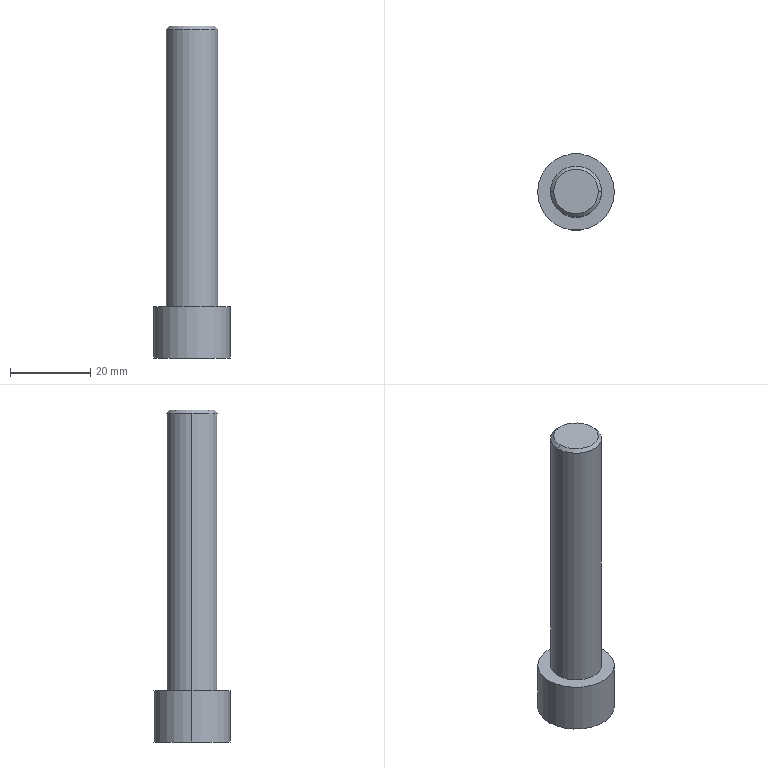Part | STEP file | 4-20.sldasm-Part-357 | 1 solid | 16 faces | box 19.05 x 19.05 x 82.55 mm | volume 11798 mm3 | plane 10 | cylinder 4 | cone 2 | commonest cylinder face diameters 12.7 x2 19.05 x2
STEP:
#1=CARTESIAN_POINT('',(90.556,-50.,63.312));
#2=VERTEX_POINT('',#1);
#3=CARTESIAN_POINT('',(79.444,-50.,63.312));
#4=VERTEX_POINT('',#3);
#5=CARTESIAN_POINT('',(85.,-50.,63.312));
#6=DIRECTION('',(0.,0.,1.));
#7=DIRECTION('',(-1.,0.,0.));
#8=AXIS2_PLACEMENT_3D('',#5,#6,#7);
#9=CIRCLE('',#8,5.556);
#10=EDGE_CURVE('',#2,#4,#9,.T.);
#11=ORIENTED_EDGE('',*,*,#10,.F.);
#12=CARTESIAN_POINT('',(91.35,-50.,62.518));
#13=VERTEX_POINT('',#12);
#14=CARTESIAN_POINT('',(91.35,-50.,62.518));
#15=DIRECTION('',(0.7071,0.,-0.7071));
#16=VECTOR('',#15,1000.);
#17=LINE('',#14,#16);
#18=EDGE_CURVE('',#2,#13,#17,.T.);
#19=ORIENTED_EDGE('',*,*,#18,.T.);
#20=CARTESIAN_POINT('',(78.65,-50.,62.518));
#21=VERTEX_POINT('',#20);
#22=CARTESIAN_POINT('',(85.,-50.,62.518));
#23=DIRECTION('',(0.,0.,-1.));
#24=DIRECTION('',(-1.,0.,0.));
#25=AXIS2_PLACEMENT_3D('',#22,#23,#24);
#26=CIRCLE('',#25,6.35);
#27=EDGE_CURVE('',#21,#13,#26,.T.);
#28=ORIENTED_EDGE('',*,*,#27,.F.);
#29=CARTESIAN_POINT('',(78.65,-50.,62.518));
#30=DIRECTION('',(-0.7071,0.,-0.7071));
#31=VECTOR('',#30,1000.);
#32=LINE('',#29,#31);
#33=EDGE_CURVE('',#4,#21,#32,.T.);
#34=ORIENTED_EDGE('',*,*,#33,.F.);
#35=EDGE_LOOP('',(#11,#19,#28,#34));
#36=FACE_OUTER_BOUND('',#35,.T.);
#37=CARTESIAN_POINT('',(85.,-50.,62.518));
#38=DIRECTION('',(0.,0.,-1.));
#39=DIRECTION('',(-1.,0.,0.));
#40=AXIS2_PLACEMENT_3D('',#37,#38,#39);
#41=CONICAL_SURFACE('',#40,6.35,0.7854);
#42=ADVANCED_FACE('',(#36),#41,.T.);
#43=CARTESIAN_POINT('',(75.475,-50.,-6.538));
#44=VERTEX_POINT('',#43);
#45=CARTESIAN_POINT('',(94.525,-50.,-6.538));
#46=VERTEX_POINT('',#45);
#47=CARTESIAN_POINT('',(85.,-50.,-6.538));
#48=DIRECTION('',(0.,0.,-1.));
#49=DIRECTION('',(-1.,0.,0.));
#50=AXIS2_PLACEMENT_3D('',#47,#48,#49);
#51=CIRCLE('',#50,9.525);
#52=EDGE_CURVE('',#44,#46,#51,.T.);
#53=ORIENTED_EDGE('',*,*,#52,.T.);
#54=CARTESIAN_POINT('',(94.525,-50.,-19.238));
#55=VERTEX_POINT('',#54);
#56=CARTESIAN_POINT('',(94.525,-50.,-6.538));
#57=DIRECTION('',(0.,0.,-1.));
#58=VECTOR('',#57,1000.);
#59=LINE('',#56,#58);
#60=EDGE_CURVE('',#46,#55,#59,.T.);
#61=ORIENTED_EDGE('',*,*,#60,.T.);
#62=CARTESIAN_POINT('',(75.475,-50.,-19.238));
#63=VERTEX_POINT('',#62);
#64=CARTESIAN_POINT('',(85.,-50.,-19.238));
#65=DIRECTION('',(0.,0.,-1.));
#66=DIRECTION('',(-1.,0.,0.));
#67=AXIS2_PLACEMENT_3D('',#64,#65,#66);
#68=CIRCLE('',#67,9.525);
#69=EDGE_CURVE('',#63,#55,#68,.T.);
#70=ORIENTED_EDGE('',*,*,#69,.F.);
#71=CARTESIAN_POINT('',(75.475,-50.,-6.538));
#72=DIRECTION('',(0.,0.,-1.));
#73=VECTOR('',#72,1000.);
#74=LINE('',#71,#73);
#75=EDGE_CURVE('',#44,#63,#74,.T.);
#76=ORIENTED_EDGE('',*,*,#75,.F.);
#77=EDGE_LOOP('',(#53,#61,#70,#76));
#78=FACE_OUTER_BOUND('',#77,.T.);
#79=CARTESIAN_POINT('',(85.,-50.,-6.538));
#80=DIRECTION('',(0.,0.,-1.));
#81=DIRECTION('',(-1.,0.,0.));
#82=AXIS2_PLACEMENT_3D('',#79,#80,#81);
#83=CYLINDRICAL_SURFACE('',#82,9.525);
#84=ADVANCED_FACE('',(#78),#83,.T.);
#85=CARTESIAN_POINT('',(78.65,-50.,-6.538));
#86=VERTEX_POINT('',#85);
#87=CARTESIAN_POINT('',(91.35,-50.,-6.538));
#88=VERTEX_POINT('',#87);
#89=CARTESIAN_POINT('',(85.,-50.,-6.538));
#90=DIRECTION('',(0.,0.,-1.));
#91=DIRECTION('',(-1.,0.,0.));
#92=AXIS2_PLACEMENT_3D('',#89,#90,#91);
#93=CIRCLE('',#92,6.35);
#94=EDGE_CURVE('',#86,#88,#93,.T.);
#95=ORIENTED_EDGE('',*,*,#94,.F.);
#96=CARTESIAN_POINT('',(78.65,-50.,-6.538));
#97=DIRECTION('',(0.,0.,1.));
#98=VECTOR('',#97,1000.);
#99=LINE('',#96,#98);
#100=EDGE_CURVE('',#86,#21,#99,.T.);
#101=ORIENTED_EDGE('',*,*,#100,.T.);
#102=ORIENTED_EDGE('',*,*,#27,.T.);
#103=CARTESIAN_POINT('',(91.35,-50.,-6.538));
#104=DIRECTION('',(0.,0.,1.));
#105=VECTOR('',#104,1000.);
#106=LINE('',#103,#105);
#107=EDGE_CURVE('',#88,#13,#106,.T.);
#108=ORIENTED_EDGE('',*,*,#107,.F.);
#109=EDGE_LOOP('',(#95,#101,#102,#108));
#110=FACE_OUTER_BOUND('',#109,.T.);
#111=CARTESIAN_POINT('',(85.,-50.,-6.538));
#112=DIRECTION('',(0.,0.,1.));
#113=DIRECTION('',(1.,0.,0.));
#114=AXIS2_PLACEMENT_3D('',#111,#112,#113);
#115=CYLINDRICAL_SURFACE('',#114,6.35);
#116=ADVANCED_FACE('',(#110),#115,.T.);
#117=ORIENTED_EDGE('',*,*,#100,.F.);
#118=CARTESIAN_POINT('',(85.,-50.,-6.538));
#119=DIRECTION('',(0.,0.,-1.));
#120=DIRECTION('',(-1.,0.,0.));
#121=AXIS2_PLACEMENT_3D('',#118,#119,#120);
#122=CIRCLE('',#121,6.35);
#123=EDGE_CURVE('',#88,#86,#122,.T.);
#124=ORIENTED_EDGE('',*,*,#123,.F.);
#125=ORIENTED_EDGE('',*,*,#107,.T.);
#126=CARTESIAN_POINT('',(85.,-50.,62.518));
#127=DIRECTION('',(0.,0.,-1.));
#128=DIRECTION('',(-1.,0.,0.));
#129=AXIS2_PLACEMENT_3D('',#126,#127,#128);
#130=CIRCLE('',#129,6.35);
#131=EDGE_CURVE('',#13,#21,#130,.T.);
#132=ORIENTED_EDGE('',*,*,#131,.T.);
#133=EDGE_LOOP('',(#117,#124,#125,#132));
#134=FACE_OUTER_BOUND('',#133,.T.);
#135=CARTESIAN_POINT('',(85.,-50.,-6.538));
#136=DIRECTION('',(0.,0.,1.));
#137=DIRECTION('',(1.,0.,0.));
#138=AXIS2_PLACEMENT_3D('',#135,#136,#137);
#139=CYLINDRICAL_SURFACE('',#138,6.35);
#140=ADVANCED_FACE('',(#134),#139,.T.);
#141=CARTESIAN_POINT('',(85.,-50.,63.312));
#142=DIRECTION('',(0.,0.,1.));
#143=DIRECTION('',(-1.,0.,0.));
#144=AXIS2_PLACEMENT_3D('',#141,#142,#143);
#145=CIRCLE('',#144,5.556);
#146=EDGE_CURVE('',#4,#2,#145,.T.);
#147=ORIENTED_EDGE('',*,*,#146,.T.);
#148=ORIENTED_EDGE('',*,*,#10,.T.);
#149=EDGE_LOOP('',(#147,#148));
#150=FACE_OUTER_BOUND('',#149,.T.);
#151=CARTESIAN_POINT('',(85.,-50.,63.312));
#152=DIRECTION('',(0.,0.,-1.));
#153=DIRECTION('',(-1.,0.,0.));
#154=AXIS2_PLACEMENT_3D('',#151,#152,#153);
#155=PLANE('',#154);
#156=ADVANCED_FACE('',(#150),#155,.F.);
#157=ORIENTED_EDGE('',*,*,#52,.F.);
#158=CARTESIAN_POINT('',(85.,-50.,-6.538));
#159=DIRECTION('',(0.,0.,-1.));
#160=DIRECTION('',(-1.,0.,0.));
#161=AXIS2_PLACEMENT_3D('',#158,#159,#160);
#162=CIRCLE('',#161,9.525);
#163=EDGE_CURVE('',#46,#44,#162,.T.);
#164=ORIENTED_EDGE('',*,*,#163,.F.);
#165=EDGE_LOOP('',(#157,#164));
#166=FACE_OUTER_BOUND('',#165,.T.);
#167=ORIENTED_EDGE('',*,*,#123,.T.);
#168=ORIENTED_EDGE('',*,*,#94,.T.);
#169=EDGE_LOOP('',(#167,#168));
#170=FACE_BOUND('',#169,.T.);
#171=CARTESIAN_POINT('',(85.,-50.,-6.538));
#172=DIRECTION('',(0.,0.,1.));
#173=DIRECTION('',(1.,0.,0.));
#174=AXIS2_PLACEMENT_3D('',#171,#172,#173);
#175=PLANE('',#174);
#176=ADVANCED_FACE('',(#166,#170),#175,.T.);
#177=CARTESIAN_POINT('',(87.75,-54.763,-19.238));
#178=VERTEX_POINT('',#177);
#179=CARTESIAN_POINT('',(82.25,-54.763,-19.238));
#180=VERTEX_POINT('',#179);
#181=CARTESIAN_POINT('',(87.75,-54.763,-19.238));
#182=DIRECTION('',(-1.,0.,0.));
#183=VECTOR('',#182,1000.);
#184=LINE('',#181,#183);
#185=EDGE_CURVE('',#178,#180,#184,.T.);
#186=ORIENTED_EDGE('',*,*,#185,.F.);
#187=CARTESIAN_POINT('',(90.499,-50.,-19.238));
#188=VERTEX_POINT('',#187);
#189=CARTESIAN_POINT('',(90.499,-50.,-19.238));
#190=DIRECTION('',(-0.5,-0.866,0.));
#191=VECTOR('',#190,1000.);
#192=LINE('',#189,#191);
#193=EDGE_CURVE('',#188,#178,#192,.T.);
#194=ORIENTED_EDGE('',*,*,#193,.F.);
#195=CARTESIAN_POINT('',(87.75,-45.238,-19.238));
#196=VERTEX_POINT('',#195);
#197=CARTESIAN_POINT('',(87.75,-45.238,-19.238));
#198=DIRECTION('',(0.5,-0.866,0.));
#199=VECTOR('',#198,1000.);
#200=LINE('',#197,#199);
#201=EDGE_CURVE('',#196,#188,#200,.T.);
#202=ORIENTED_EDGE('',*,*,#201,.F.);
#203=CARTESIAN_POINT('',(82.25,-45.238,-19.238));
#204=VERTEX_POINT('',#203);
#205=CARTESIAN_POINT('',(82.25,-45.238,-19.238));
#206=DIRECTION('',(1.,0.,0.));
#207=VECTOR('',#206,1000.);
#208=LINE('',#205,#207);
#209=EDGE_CURVE('',#204,#196,#208,.T.);
#210=ORIENTED_EDGE('',*,*,#209,.F.);
#211=CARTESIAN_POINT('',(79.501,-50.,-19.238));
#212=VERTEX_POINT('',#211);
#213=CARTESIAN_POINT('',(79.501,-50.,-19.238));
#214=DIRECTION('',(0.5,0.866,0.));
#215=VECTOR('',#214,1000.);
#216=LINE('',#213,#215);
#217=EDGE_CURVE('',#212,#204,#216,.T.);
#218=ORIENTED_EDGE('',*,*,#217,.F.);
#219=CARTESIAN_POINT('',(82.25,-54.763,-19.238));
#220=DIRECTION('',(-0.5,0.866,0.));
#221=VECTOR('',#220,1000.);
#222=LINE('',#219,#221);
#223=EDGE_CURVE('',#180,#212,#222,.T.);
#224=ORIENTED_EDGE('',*,*,#223,.F.);
#225=EDGE_LOOP('',(#186,#194,#202,#210,#218,#224));
#226=FACE_BOUND('',#225,.T.);
#227=ORIENTED_EDGE('',*,*,#69,.T.);
#228=CARTESIAN_POINT('',(85.,-50.,-19.238));
#229=DIRECTION('',(0.,0.,-1.));
#230=DIRECTION('',(-1.,0.,0.));
#231=AXIS2_PLACEMENT_3D('',#228,#229,#230);
#232=CIRCLE('',#231,9.525);
#233=EDGE_CURVE('',#55,#63,#232,.T.);
#234=ORIENTED_EDGE('',*,*,#233,.T.);
#235=EDGE_LOOP('',(#227,#234));
#236=FACE_OUTER_BOUND('',#235,.T.);
#237=CARTESIAN_POINT('',(85.,-50.,-19.238));
#238=DIRECTION('',(0.,0.,-1.));
#239=DIRECTION('',(-1.,0.,0.));
#240=AXIS2_PLACEMENT_3D('',#237,#238,#239);
#241=PLANE('',#240);
#242=ADVANCED_FACE('',(#226,#236),#241,.T.);
#243=ORIENTED_EDGE('',*,*,#60,.F.);
#244=ORIENTED_EDGE('',*,*,#163,.T.);
#245=ORIENTED_EDGE('',*,*,#75,.T.);
#246=ORIENTED_EDGE('',*,*,#233,.F.);
#247=EDGE_LOOP('',(#243,#244,#245,#246));
#248=FACE_OUTER_BOUND('',#247,.T.);
#249=CARTESIAN_POINT('',(85.,-50.,-6.538));
#250=DIRECTION('',(0.,0.,-1.));
#251=DIRECTION('',(-1.,0.,0.));
#252=AXIS2_PLACEMENT_3D('',#249,#250,#251);
#253=CYLINDRICAL_SURFACE('',#252,9.525);
#254=ADVANCED_FACE('',(#248),#253,.T.);
#255=ORIENTED_EDGE('',*,*,#18,.F.);
#256=ORIENTED_EDGE('',*,*,#146,.F.);
#257=ORIENTED_EDGE('',*,*,#33,.T.);
#258=ORIENTED_EDGE('',*,*,#131,.F.);
#259=EDGE_LOOP('',(#255,#256,#257,#258));
#260=FACE_OUTER_BOUND('',#259,.T.);
#261=CARTESIAN_POINT('',(85.,-50.,62.518));
#262=DIRECTION('',(0.,0.,-1.));
#263=DIRECTION('',(-1.,0.,0.));
#264=AXIS2_PLACEMENT_3D('',#261,#262,#263);
#265=CONICAL_SURFACE('',#264,6.35,0.7854);
#266=ADVANCED_FACE('',(#260),#265,.T.);
#267=ORIENTED_EDGE('',*,*,#185,.T.);
#268=CARTESIAN_POINT('',(82.25,-54.763,-10.856));
#269=VERTEX_POINT('',#268);
#270=CARTESIAN_POINT('',(82.25,-54.763,-10.856));
#271=DIRECTION('',(0.,0.,-1.));
#272=VECTOR('',#271,1000.);
#273=LINE('',#270,#272);
#274=EDGE_CURVE('',#269,#180,#273,.T.);
#275=ORIENTED_EDGE('',*,*,#274,.F.);
#276=CARTESIAN_POINT('',(87.75,-54.763,-10.856));
#277=VERTEX_POINT('',#276);
#278=CARTESIAN_POINT('',(87.75,-54.763,-10.856));
#279=DIRECTION('',(-1.,0.,0.));
#280=VECTOR('',#279,1000.);
#281=LINE('',#278,#280);
#282=EDGE_CURVE('',#277,#269,#281,.T.);
#283=ORIENTED_EDGE('',*,*,#282,.F.);
#284=CARTESIAN_POINT('',(87.75,-54.763,-10.856));
#285=DIRECTION('',(0.,0.,-1.));
#286=VECTOR('',#285,1000.);
#287=LINE('',#284,#286);
#288=EDGE_CURVE('',#277,#178,#287,.T.);
#289=ORIENTED_EDGE('',*,*,#288,.T.);
#290=EDGE_LOOP('',(#267,#275,#283,#289));
#291=FACE_OUTER_BOUND('',#290,.T.);
#292=CARTESIAN_POINT('',(87.75,-54.763,-10.856));
#293=DIRECTION('',(0.,-1.,0.));
#294=DIRECTION('',(0.,0.,1.));
#295=AXIS2_PLACEMENT_3D('',#292,#293,#294);
#296=PLANE('',#295);
#297=ADVANCED_FACE('',(#291),#296,.F.);
#298=ORIENTED_EDGE('',*,*,#223,.T.);
#299=CARTESIAN_POINT('',(79.501,-50.,-10.856));
#300=VERTEX_POINT('',#299);
#301=CARTESIAN_POINT('',(79.501,-50.,-10.856));
#302=DIRECTION('',(0.,0.,-1.));
#303=VECTOR('',#302,1000.);
#304=LINE('',#301,#303);
#305=EDGE_CURVE('',#300,#212,#304,.T.);
#306=ORIENTED_EDGE('',*,*,#305,.F.);
#307=CARTESIAN_POINT('',(82.25,-54.763,-10.856));
#308=DIRECTION('',(-0.5,0.866,0.));
#309=VECTOR('',#308,1000.);
#310=LINE('',#307,#309);
#311=EDGE_CURVE('',#269,#300,#310,.T.);
#312=ORIENTED_EDGE('',*,*,#311,.F.);
#313=ORIENTED_EDGE('',*,*,#274,.T.);
#314=EDGE_LOOP('',(#298,#306,#312,#313));
#315=FACE_OUTER_BOUND('',#314,.T.);
#316=CARTESIAN_POINT('',(82.25,-54.763,-10.856));
#317=DIRECTION('',(-0.866,-0.5,0.));
#318=DIRECTION('',(-0.5,0.866,0.));
#319=AXIS2_PLACEMENT_3D('',#316,#317,#318);
#320=PLANE('',#319);
#321=ADVANCED_FACE('',(#315),#320,.F.);
#322=ORIENTED_EDGE('',*,*,#217,.T.);
#323=CARTESIAN_POINT('',(82.25,-45.238,-10.856));
#324=VERTEX_POINT('',#323);
#325=CARTESIAN_POINT('',(82.25,-45.238,-10.856));
#326=DIRECTION('',(0.,0.,-1.));
#327=VECTOR('',#326,1000.);
#328=LINE('',#325,#327);
#329=EDGE_CURVE('',#324,#204,#328,.T.);
#330=ORIENTED_EDGE('',*,*,#329,.F.);
#331=CARTESIAN_POINT('',(79.501,-50.,-10.856));
#332=DIRECTION('',(0.5,0.866,0.));
#333=VECTOR('',#332,1000.);
#334=LINE('',#331,#333);
#335=EDGE_CURVE('',#300,#324,#334,.T.);
#336=ORIENTED_EDGE('',*,*,#335,.F.);
#337=ORIENTED_EDGE('',*,*,#305,.T.);
#338=EDGE_LOOP('',(#322,#330,#336,#337));
#339=FACE_OUTER_BOUND('',#338,.T.);
#340=CARTESIAN_POINT('',(79.501,-50.,-10.856));
#341=DIRECTION('',(-0.866,0.5,0.));
#342=DIRECTION('',(0.5,0.866,0.));
#343=AXIS2_PLACEMENT_3D('',#340,#341,#342);
#344=PLANE('',#343);
#345=ADVANCED_FACE('',(#339),#344,.F.);
#346=ORIENTED_EDGE('',*,*,#209,.T.);
#347=CARTESIAN_POINT('',(87.75,-45.238,-10.856));
#348=VERTEX_POINT('',#347);
#349=CARTESIAN_POINT('',(87.75,-45.238,-10.856));
#350=DIRECTION('',(0.,0.,-1.));
#351=VECTOR('',#350,1000.);
#352=LINE('',#349,#351);
#353=EDGE_CURVE('',#348,#196,#352,.T.);
#354=ORIENTED_EDGE('',*,*,#353,.F.);
#355=CARTESIAN_POINT('',(82.25,-45.238,-10.856));
#356=DIRECTION('',(1.,0.,0.));
#357=VECTOR('',#356,1000.);
#358=LINE('',#355,#357);
#359=EDGE_CURVE('',#324,#348,#358,.T.);
#360=ORIENTED_EDGE('',*,*,#359,.F.);
#361=ORIENTED_EDGE('',*,*,#329,.T.);
#362=EDGE_LOOP('',(#346,#354,#360,#361));
#363=FACE_OUTER_BOUND('',#362,.T.);
#364=CARTESIAN_POINT('',(82.25,-45.238,-10.856));
#365=DIRECTION('',(0.,1.,0.));
#366=DIRECTION('',(0.,0.,-1.));
#367=AXIS2_PLACEMENT_3D('',#364,#365,#366);
#368=PLANE('',#367);
#369=ADVANCED_FACE('',(#363),#368,.F.);
#370=ORIENTED_EDGE('',*,*,#201,.T.);
#371=CARTESIAN_POINT('',(90.499,-50.,-10.856));
#372=VERTEX_POINT('',#371);
#373=CARTESIAN_POINT('',(90.499,-50.,-10.856));
#374=DIRECTION('',(0.,0.,-1.));
#375=VECTOR('',#374,1000.);
#376=LINE('',#373,#375);
#377=EDGE_CURVE('',#372,#188,#376,.T.);
#378=ORIENTED_EDGE('',*,*,#377,.F.);
#379=CARTESIAN_POINT('',(87.75,-45.238,-10.856));
#380=DIRECTION('',(0.5,-0.866,0.));
#381=VECTOR('',#380,1000.);
#382=LINE('',#379,#381);
#383=EDGE_CURVE('',#348,#372,#382,.T.);
#384=ORIENTED_EDGE('',*,*,#383,.F.);
#385=ORIENTED_EDGE('',*,*,#353,.T.);
#386=EDGE_LOOP('',(#370,#378,#384,#385));
#387=FACE_OUTER_BOUND('',#386,.T.);
#388=CARTESIAN_POINT('',(87.75,-45.238,-10.856));
#389=DIRECTION('',(0.866,0.5,0.));
#390=DIRECTION('',(0.5,-0.866,0.));
#391=AXIS2_PLACEMENT_3D('',#388,#389,#390);
#392=PLANE('',#391);
#393=ADVANCED_FACE('',(#387),#392,.F.);
#394=ORIENTED_EDGE('',*,*,#193,.T.);
#395=ORIENTED_EDGE('',*,*,#288,.F.);
#396=CARTESIAN_POINT('',(90.499,-50.,-10.856));
#397=DIRECTION('',(-0.5,-0.866,0.));
#398=VECTOR('',#397,1000.);
#399=LINE('',#396,#398);
#400=EDGE_CURVE('',#372,#277,#399,.T.);
#401=ORIENTED_EDGE('',*,*,#400,.F.);
#402=ORIENTED_EDGE('',*,*,#377,.T.);
#403=EDGE_LOOP('',(#394,#395,#401,#402));
#404=FACE_OUTER_BOUND('',#403,.T.);
#405=CARTESIAN_POINT('',(90.499,-50.,-10.856));
#406=DIRECTION('',(0.866,-0.5,0.));
#407=DIRECTION('',(-0.5,-0.866,0.));
#408=AXIS2_PLACEMENT_3D('',#405,#406,#407);
#409=PLANE('',#408);
#410=ADVANCED_FACE('',(#404),#409,.F.);
#411=ORIENTED_EDGE('',*,*,#282,.T.);
#412=ORIENTED_EDGE('',*,*,#311,.T.);
#413=ORIENTED_EDGE('',*,*,#335,.T.);
#414=ORIENTED_EDGE('',*,*,#359,.T.);
#415=ORIENTED_EDGE('',*,*,#383,.T.);
#416=ORIENTED_EDGE('',*,*,#400,.T.);
#417=EDGE_LOOP('',(#411,#412,#413,#414,#415,#416));
#418=FACE_OUTER_BOUND('',#417,.T.);
#419=CARTESIAN_POINT('',(82.25,-54.763,-10.856));
#420=DIRECTION('',(0.,0.,-1.));
#421=DIRECTION('',(-1.,0.,0.));
#422=AXIS2_PLACEMENT_3D('',#419,#420,#421);
#423=PLANE('',#422);
#424=ADVANCED_FACE('',(#418),#423,.T.);
#425=CLOSED_SHELL('',(#42,#84,#116,#140,#156,#176,#242,#254,#266,#297,#321,#345,#369,#393,#410,#424));
#426=MANIFOLD_SOLID_BREP('',#425);
#427=CARTESIAN_POINT('',(0.,0.,0.));
#428=DIRECTION('',(0.,0.,1.));
#429=DIRECTION('',(1.,0.,0.));
#430=AXIS2_PLACEMENT_3D('',#427,#428,#429);
#431=(LENGTH_UNIT()NAMED_UNIT(*)SI_UNIT(.MILLI.,.METRE.));
#432=UNCERTAINTY_MEASURE_WITH_UNIT(LENGTH_MEASURE(0.00001),#431,'','');
#433=(NAMED_UNIT(*)PLANE_ANGLE_UNIT()SI_UNIT($,.RADIAN.));
#434=(NAMED_UNIT(*)SI_UNIT($,.STERADIAN.)SOLID_ANGLE_UNIT());
#435=(GEOMETRIC_REPRESENTATION_CONTEXT(3)GLOBAL_UNCERTAINTY_ASSIGNED_CONTEXT((#432))GLOBAL_UNIT_ASSIGNED_CONTEXT((#431,#433,#434))REPRESENTATION_CONTEXT('',''));
#436=ADVANCED_BREP_SHAPE_REPRESENTATION('',(#426,#430),#435);